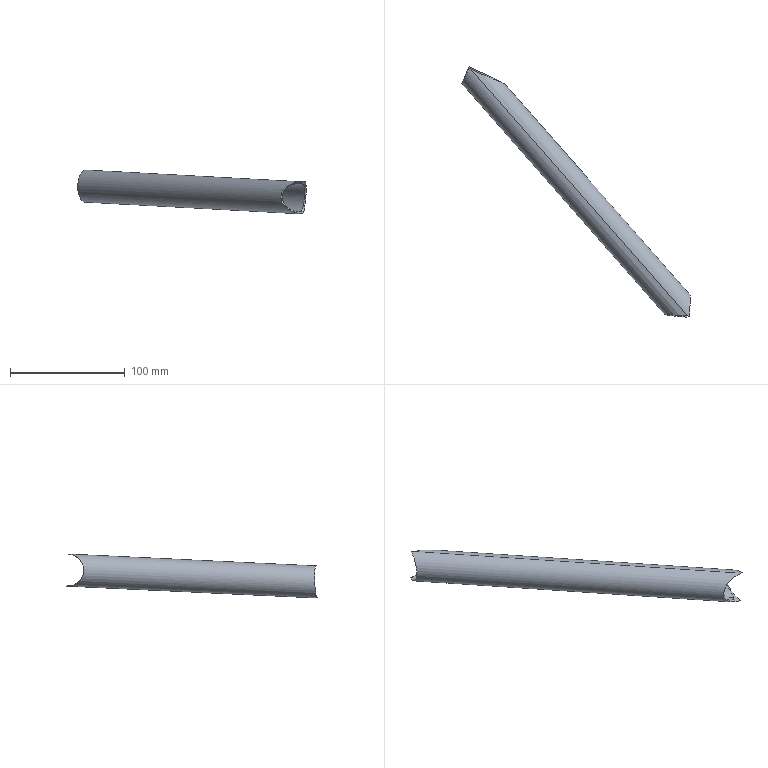Part | STEP file | PRT0001_68_15 | 1 solid | 6 faces | box 199.467 x 218.482 x 38.316 mm | volume 33314 mm3 | cylinder 6 | commonest cylinder face diameters 28 x4 25 x2